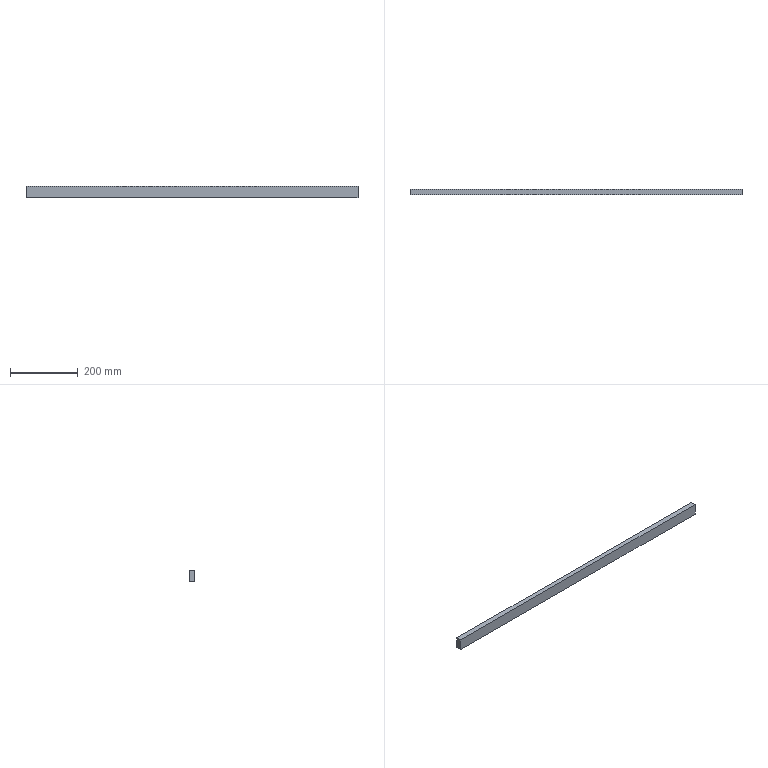Part | NX | features BREP 1 | 1 solid | 6 faces | box 977.78 x 15 x 35 mm | volume 513334 mm3 | plane 6
STEP:
#1=CARTESIAN_POINT('',(687.678,-679.988,100.));
#2=VERTEX_POINT('',#1);
#3=CARTESIAN_POINT('',(687.678,-679.988,65.));
#4=VERTEX_POINT('',#3);
#5=CARTESIAN_POINT('',(687.678,-679.988,82.5));
#6=DIRECTION('',(0.,0.,-1.));
#7=VECTOR('',#6,1000.);
#8=LINE('',#5,#7);
#9=EDGE_CURVE('',#2,#4,#8,.T.);
#10=ORIENTED_EDGE('',*,*,#9,.F.);
#11=CARTESIAN_POINT('',(687.678,-664.988,100.));
#12=VERTEX_POINT('',#11);
#13=CARTESIAN_POINT('',(687.678,-672.488,100.));
#14=DIRECTION('',(0.,1.,0.));
#15=VECTOR('',#14,1000.);
#16=LINE('',#13,#15);
#17=EDGE_CURVE('',#2,#12,#16,.T.);
#18=ORIENTED_EDGE('',*,*,#17,.T.);
#19=CARTESIAN_POINT('',(687.678,-664.988,65.));
#20=VERTEX_POINT('',#19);
#21=CARTESIAN_POINT('',(687.678,-664.988,82.5));
#22=DIRECTION('',(0.,0.,-1.));
#23=VECTOR('',#22,1000.);
#24=LINE('',#21,#23);
#25=EDGE_CURVE('',#12,#20,#24,.T.);
#26=ORIENTED_EDGE('',*,*,#25,.T.);
#27=CARTESIAN_POINT('',(687.678,-672.488,65.));
#28=DIRECTION('',(0.,1.,0.));
#29=VECTOR('',#28,1000.);
#30=LINE('',#27,#29);
#31=EDGE_CURVE('',#4,#20,#30,.T.);
#32=ORIENTED_EDGE('',*,*,#31,.F.);
#33=EDGE_LOOP('',(#10,#18,#26,#32));
#34=FACE_BOUND('',#33,.T.);
#35=CARTESIAN_POINT('',(687.678,-679.988,82.5));
#36=DIRECTION('',(-1.,0.,0.));
#37=DIRECTION('',(0.,1.,0.));
#38=AXIS2_PLACEMENT_3D('',#35,#36,#37);
#39=PLANE('',#38);
#40=ADVANCED_FACE('',(#34),#39,.T.);
#41=CARTESIAN_POINT('',(1665.458,-679.988,100.));
#42=VERTEX_POINT('',#41);
#43=CARTESIAN_POINT('',(1665.458,-679.988,65.));
#44=VERTEX_POINT('',#43);
#45=CARTESIAN_POINT('',(1665.458,-679.988,82.5));
#46=DIRECTION('',(0.,0.,-1.));
#47=VECTOR('',#46,1000.);
#48=LINE('',#45,#47);
#49=EDGE_CURVE('',#42,#44,#48,.T.);
#50=ORIENTED_EDGE('',*,*,#49,.F.);
#51=CARTESIAN_POINT('',(1176.568,-679.988,100.));
#52=DIRECTION('',(1.,0.,0.));
#53=VECTOR('',#52,1000.);
#54=LINE('',#51,#53);
#55=EDGE_CURVE('',#2,#42,#54,.T.);
#56=ORIENTED_EDGE('',*,*,#55,.F.);
#57=ORIENTED_EDGE('',*,*,#9,.T.);
#58=CARTESIAN_POINT('',(1176.568,-679.988,65.));
#59=DIRECTION('',(1.,0.,0.));
#60=VECTOR('',#59,1000.);
#61=LINE('',#58,#60);
#62=EDGE_CURVE('',#4,#44,#61,.T.);
#63=ORIENTED_EDGE('',*,*,#62,.T.);
#64=EDGE_LOOP('',(#50,#56,#57,#63));
#65=FACE_BOUND('',#64,.T.);
#66=CARTESIAN_POINT('',(642.389,-679.988,95.));
#67=DIRECTION('',(0.,1.,0.));
#68=DIRECTION('',(0.,0.,-1.));
#69=AXIS2_PLACEMENT_3D('',#66,#67,#68);
#70=PLANE('',#69);
#71=ADVANCED_FACE('',(#65),#70,.F.);
#72=CARTESIAN_POINT('',(1665.458,-664.988,100.));
#73=VERTEX_POINT('',#72);
#74=CARTESIAN_POINT('',(1665.458,-672.488,100.));
#75=DIRECTION('',(0.,-1.,0.));
#76=VECTOR('',#75,1000.);
#77=LINE('',#74,#76);
#78=EDGE_CURVE('',#73,#42,#77,.T.);
#79=ORIENTED_EDGE('',*,*,#78,.F.);
#80=CARTESIAN_POINT('',(1176.568,-664.988,100.));
#81=DIRECTION('',(-1.,0.,0.));
#82=VECTOR('',#81,1000.);
#83=LINE('',#80,#82);
#84=EDGE_CURVE('',#73,#12,#83,.T.);
#85=ORIENTED_EDGE('',*,*,#84,.T.);
#86=ORIENTED_EDGE('',*,*,#17,.F.);
#87=ORIENTED_EDGE('',*,*,#55,.T.);
#88=EDGE_LOOP('',(#79,#85,#86,#87));
#89=FACE_BOUND('',#88,.T.);
#90=CARTESIAN_POINT('',(1176.568,-679.988,100.));
#91=DIRECTION('',(0.,0.,-1.));
#92=DIRECTION('',(1.,0.,0.));
#93=AXIS2_PLACEMENT_3D('',#90,#91,#92);
#94=PLANE('',#93);
#95=ADVANCED_FACE('',(#89),#94,.F.);
#96=CARTESIAN_POINT('',(1665.458,-664.988,65.));
#97=VERTEX_POINT('',#96);
#98=CARTESIAN_POINT('',(1176.568,-664.988,65.));
#99=DIRECTION('',(-1.,0.,0.));
#100=VECTOR('',#99,1000.);
#101=LINE('',#98,#100);
#102=EDGE_CURVE('',#97,#20,#101,.T.);
#103=ORIENTED_EDGE('',*,*,#102,.T.);
#104=ORIENTED_EDGE('',*,*,#25,.F.);
#105=ORIENTED_EDGE('',*,*,#84,.F.);
#106=CARTESIAN_POINT('',(1665.458,-664.988,82.5));
#107=DIRECTION('',(0.,0.,-1.));
#108=VECTOR('',#107,1000.);
#109=LINE('',#106,#108);
#110=EDGE_CURVE('',#73,#97,#109,.T.);
#111=ORIENTED_EDGE('',*,*,#110,.T.);
#112=EDGE_LOOP('',(#103,#104,#105,#111));
#113=FACE_BOUND('',#112,.T.);
#114=CARTESIAN_POINT('',(642.389,-664.988,95.));
#115=DIRECTION('',(0.,1.,0.));
#116=DIRECTION('',(0.,0.,-1.));
#117=AXIS2_PLACEMENT_3D('',#114,#115,#116);
#118=PLANE('',#117);
#119=ADVANCED_FACE('',(#113),#118,.T.);
#120=ORIENTED_EDGE('',*,*,#62,.F.);
#121=ORIENTED_EDGE('',*,*,#31,.T.);
#122=ORIENTED_EDGE('',*,*,#102,.F.);
#123=CARTESIAN_POINT('',(1665.458,-672.488,65.));
#124=DIRECTION('',(0.,-1.,0.));
#125=VECTOR('',#124,1000.);
#126=LINE('',#123,#125);
#127=EDGE_CURVE('',#97,#44,#126,.T.);
#128=ORIENTED_EDGE('',*,*,#127,.T.);
#129=EDGE_LOOP('',(#120,#121,#122,#128));
#130=FACE_BOUND('',#129,.T.);
#131=CARTESIAN_POINT('',(1176.568,-679.988,65.));
#132=DIRECTION('',(0.,0.,-1.));
#133=DIRECTION('',(1.,0.,0.));
#134=AXIS2_PLACEMENT_3D('',#131,#132,#133);
#135=PLANE('',#134);
#136=ADVANCED_FACE('',(#130),#135,.T.);
#137=ORIENTED_EDGE('',*,*,#127,.F.);
#138=ORIENTED_EDGE('',*,*,#110,.F.);
#139=ORIENTED_EDGE('',*,*,#78,.T.);
#140=ORIENTED_EDGE('',*,*,#49,.T.);
#141=EDGE_LOOP('',(#137,#138,#139,#140));
#142=FACE_BOUND('',#141,.T.);
#143=CARTESIAN_POINT('',(1665.458,-679.988,82.5));
#144=DIRECTION('',(-1.,0.,0.));
#145=DIRECTION('',(0.,1.,0.));
#146=AXIS2_PLACEMENT_3D('',#143,#144,#145);
#147=PLANE('',#146);
#148=ADVANCED_FACE('',(#142),#147,.F.);
#149=CLOSED_SHELL('',(#40,#71,#95,#119,#136,#148));
#150=MANIFOLD_SOLID_BREP('',#149);
#151=(LENGTH_UNIT()NAMED_UNIT(*)SI_UNIT(.MILLI.,.METRE.));
#152=UNCERTAINTY_MEASURE_WITH_UNIT(LENGTH_MEASURE(0.00001),#151,'','');
#153=(NAMED_UNIT(*)PLANE_ANGLE_UNIT()SI_UNIT($,.RADIAN.));
#154=(NAMED_UNIT(*)SI_UNIT($,.STERADIAN.)SOLID_ANGLE_UNIT());
#155=(GEOMETRIC_REPRESENTATION_CONTEXT(3)GLOBAL_UNCERTAINTY_ASSIGNED_CONTEXT((#152))GLOBAL_UNIT_ASSIGNED_CONTEXT((#151,#153,#154))REPRESENTATION_CONTEXT('',''));
#156=ADVANCED_BREP_SHAPE_REPRESENTATION('',(#150),#155);